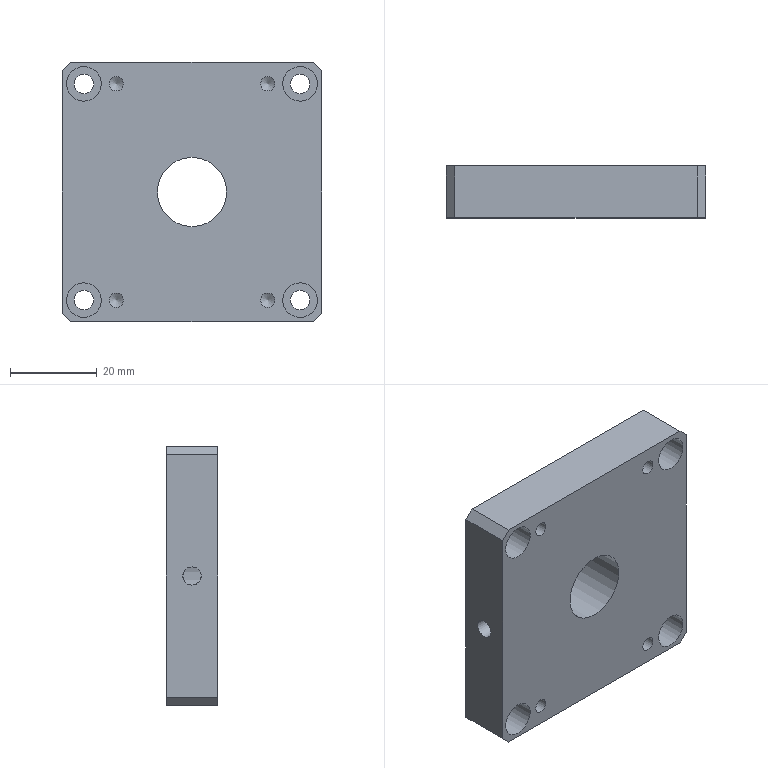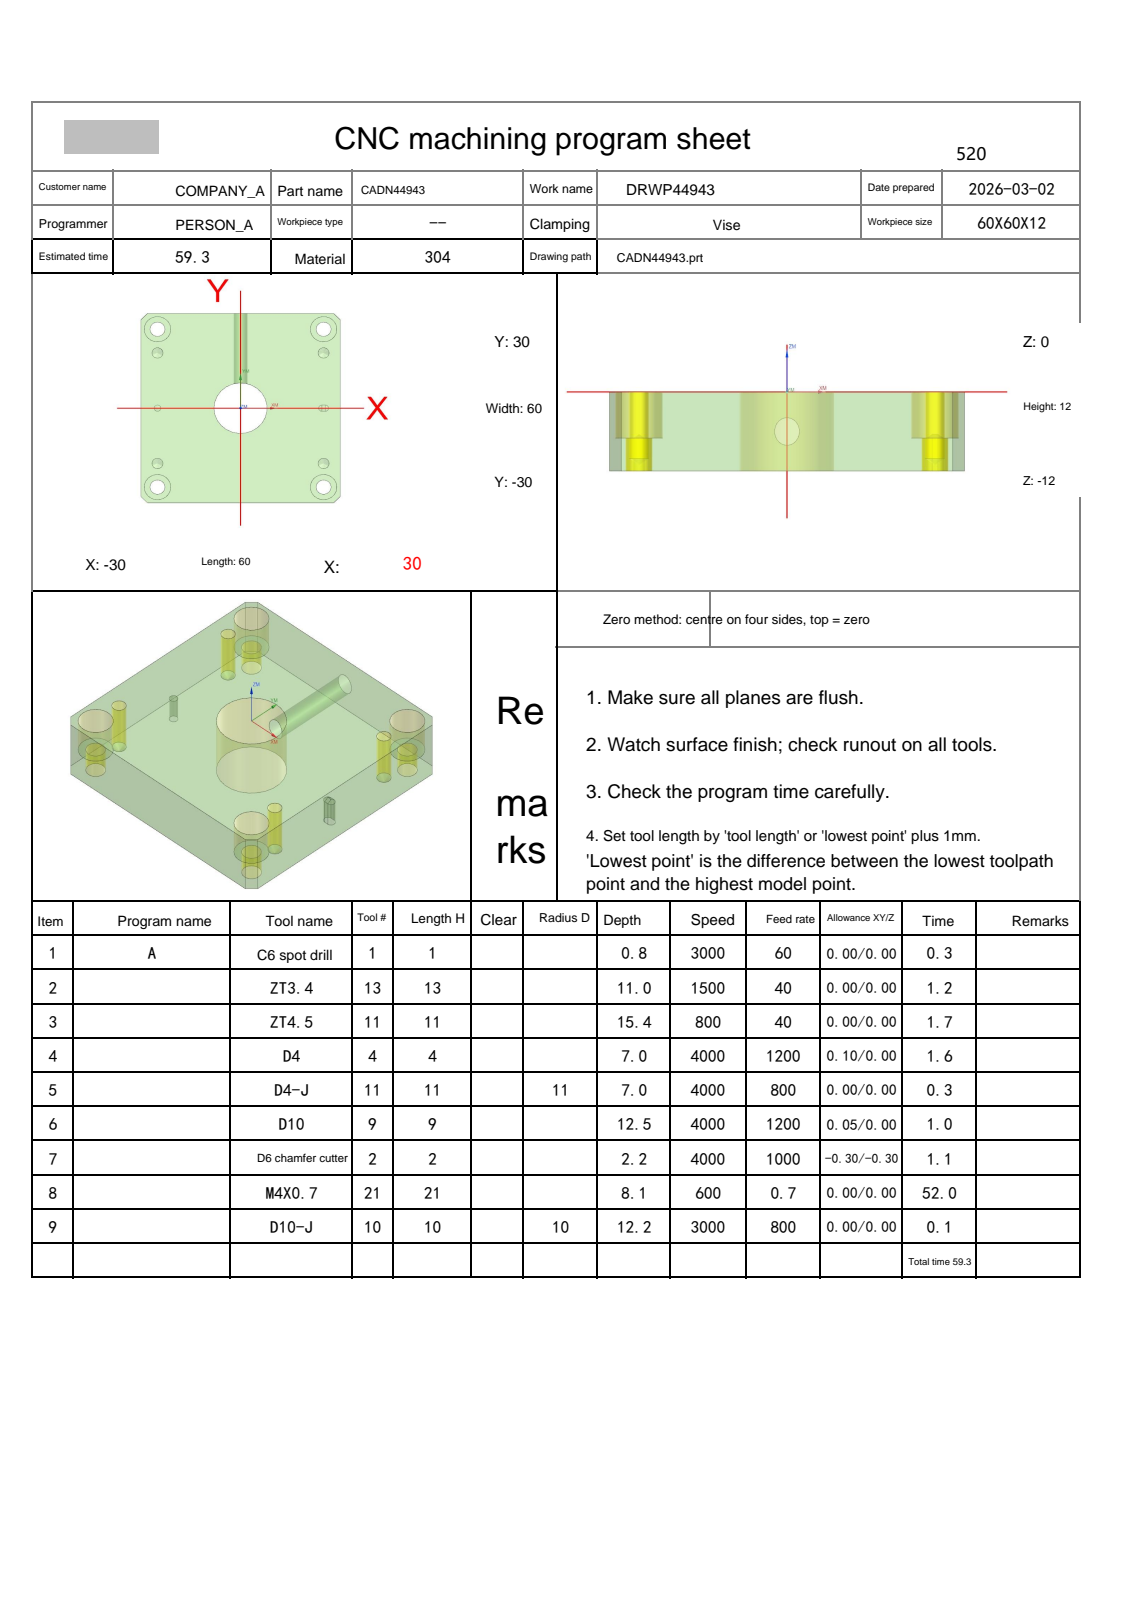NC program | NX | posted by the shop | part box 60 x 12 x 60 mm
Whole program:
%
O0001
(Machine time: 107.25 MIN)
(===Total Tool:8===)
(T1=C6 spot drill   D=6.   R=0.   D-  H01 Z=-0.8  )
(T13=ZT3.4  D=3.4  DR_a=118 D-  H13 Z=-11.  )
(T11=ZT4.5  D=4.5  DR_a=118 D-  H11 Z=-15.35)
(T4=D4      D=4.   R=0.   D-  H04 Z=-7.   )
(T9=D10     D=10.  R=0.   D-  H09 Z=-12.5 )
(T2=D6 chamfer cutter   D=6.   R=0.   D-  H02 Z=-2.2  )
(T21=M4X0.7 D=3.3  DR_a=180 D-  H21 Z=-8.1  )
(T10=D10-J  D=10.  R=0.   D10 H10 Z=-12.2 )
G80 G90 G17 G49 G40
G91 G28 Z0
M01
N1 T01 M06
(C6 spot drill  D=6. R=0. H=01 ce=0.00 di=0.00)
G00 G90 G54 X25. Y25. M03 S3000
G43 H01 Z50.
M08
G98 G81 X25. Y25. Z-.8 R1. F60.
Y17.5
Y-17.5
Y-25.
X0.0 Y0.0
X-25. Y25.
Y17.5
Y-17.5
Y-25.
G80
G00 Z50.
G91 G28 Z0.0
M05
M09
G91 G28 Z0.0
M01
N2 T13 M06
(ZT3.4 D=3.4 DR_a=118 H=13)
G00 G90 G54 X25. Y17.5 M03 S1500
G43 H13 Z50.
M08
G98 G83 X25. Y17.5 Z-11. R1. F40. Q1.
Y-17.5
X-25.
Y17.5
G80
G00 Z50.
G91 G28 Z0.0
M05
M09
G91 G28 Z0.0
M01
N3 T11 M06
(ZT4.5 D=4.5 DR_a=118 H=11)
G00 G90 G54 X-25. Y-25. M03 S800
G43 H11 Z50.
M08
G98 G83 X-25. Y-25. Z-15.352 R1. F40. Q1.
Y25.
X25.
Y-25.
G80
G00 Z50.
G91 G28 Z0.0
M05
M09
G91 G28 Z0.0
M01
N4 T04 M06
(D4  D=4. R=0. H=04 ce=0.10 di=0.00)
G00 G90 G54 X-25. Y-25. M03 S4000
G43 H04 Z50.
M08
Z.5
G03 X-25.95 Y-25.95 I0.0 J-.95 F1200.
X-25. Y-26.9 I.95 J0.0
X-25. Y-26.9 Z.3 I0.0 J1.9
X-25. Y-26.9 Z.1 I0.0 J1.9
X-25. Y-26.9 Z-.1 I0.0 J1.9
X-25. Y-26.9 Z-.3 I0.0 J1.9
X-25. Y-26.9 Z-.5 I0.0 J1.9
X-25. Y-26.9 Z-.7 I0.0 J1.9
X-25. Y-26.9 Z-.9 I0.0 J1.9
X-25. Y-26.9 Z-1.1 I0.0 J1.9
X-25. Y-26.9 Z-1.3 I0.0 J1.9
X-25. Y-26.9 Z-1.5 I0.0 J1.9
X-25. Y-26.9 Z-1.7 I0.0 J1.9
X-25. Y-26.9 Z-1.9 I0.0 J1.9
X-25. Y-26.9 Z-2.1 I0.0 J1.9
X-25. Y-26.9 Z-2.3 I0.0 J1.9
X-25. Y-26.9 Z-2.5 I0.0 J1.9
X-25. Y-26.9 Z-2.7 I0.0 J1.9
X-25. Y-26.9 Z-2.9 I0.0 J1.9
X-25. Y-26.9 Z-3.1 I0.0 J1.9
X-25. Y-26.9 Z-3.3 I0.0 J1.9
X-25. Y-26.9 Z-3.5 I0.0 J1.9
X-25. Y-26.9 Z-3.7 I0.0 J1.9
X-25. Y-26.9 Z-3.9 I0.0 J1.9
X-25. Y-26.9 Z-4.1 I0.0 J1.9
X-25. Y-26.9 Z-4.3 I0.0 J1.9
X-25. Y-26.9 Z-4.5 I0.0 J1.9
X-25. Y-26.9 Z-4.7 I0.0 J1.9
X-25. Y-26.9 Z-4.9 I0.0 J1.9
X-25. Y-26.9 Z-5.1 I0.0 J1.9
X-25. Y-26.9 Z-5.3 I0.0 J1.9
X-25. Y-26.9 Z-5.5 I0.0 J1.9
X-25. Y-26.9 Z-5.7 I0.0 J1.9
X-25. Y-26.9 Z-5.9 I0.0 J1.9
X-25. Y-26.9 Z-6.1 I0.0 J1.9
X-25. Y-26.9 Z-6.3 I0.0 J1.9
X-25. Y-26.9 Z-6.5 I0.0 J1.9
X-25. Y-26.9 Z-6.7 I0.0 J1.9
X-25. Y-26.9 Z-6.9 I0.0 J1.9
X-25. Y-23.1 Z-7. I0.0 J1.9
X-26.9 Y-25. I0.0 J-1.9
X-25. Y-26.9 I1.9 J0.0
X-23.1 Y-25. I0.0 J1.9
X-25. Y-23.1 I-1.9 J0.0
X-25.95 Y-24.05 I0.0 J-.95
X-25. Y-25. I.95 J0.0
G00 Z50.
Y25.
Z.5
G03 X-25.95 Y24.05 I0.0 J-.95
X-25. Y23.1 I.95 J0.0
X-25. Y23.1 Z.3 I0.0 J1.9
X-25. Y23.1 Z.1 I0.0 J1.9
X-25. Y23.1 Z-.1 I0.0 J1.9
X-25. Y23.1 Z-.3 I0.0 J1.9
X-25. Y23.1 Z-.5 I0.0 J1.9
X-25. Y23.1 Z-.7 I0.0 J1.9
X-25. Y23.1 Z-.9 I0.0 J1.9
X-25. Y23.1 Z-1.1 I0.0 J1.9
X-25. Y23.1 Z-1.3 I0.0 J1.9
X-25. Y23.1 Z-1.5 I0.0 J1.9
X-25. Y23.1 Z-1.7 I0.0 J1.9
X-25. Y23.1 Z-1.9 I0.0 J1.9
X-25. Y23.1 Z-2.1 I0.0 J1.9
X-25. Y23.1 Z-2.3 I0.0 J1.9
X-25. Y23.1 Z-2.5 I0.0 J1.9
X-25. Y23.1 Z-2.7 I0.0 J1.9
X-25. Y23.1 Z-2.9 I0.0 J1.9
X-25. Y23.1 Z-3.1 I0.0 J1.9
X-25. Y23.1 Z-3.3 I0.0 J1.9
X-25. Y23.1 Z-3.5 I0.0 J1.9
X-25. Y23.1 Z-3.7 I0.0 J1.9
X-25. Y23.1 Z-3.9 I0.0 J1.9
X-25. Y23.1 Z-4.1 I0.0 J1.9
X-25. Y23.1 Z-4.3 I0.0 J1.9
X-25. Y23.1 Z-4.5 I0.0 J1.9
X-25. Y23.1 Z-4.7 I0.0 J1.9
X-25. Y23.1 Z-4.9 I0.0 J1.9
X-25. Y23.1 Z-5.1 I0.0 J1.9
X-25. Y23.1 Z-5.3 I0.0 J1.9
X-25. Y23.1 Z-5.5 I0.0 J1.9
X-25. Y23.1 Z-5.7 I0.0 J1.9
X-25. Y23.1 Z-5.9 I0.0 J1.9
X-25. Y23.1 Z-6.1 I0.0 J1.9
X-25. Y23.1 Z-6.3 I0.0 J1.9
X-25. Y23.1 Z-6.5 I0.0 J1.9
X-25. Y23.1 Z-6.7 I0.0 J1.9
X-25. Y23.1 Z-6.9 I0.0 J1.9
X-25. Y26.9 Z-7. I0.0 J1.9
X-26.9 Y25. I0.0 J-1.9
X-25. Y23.1 I1.9 J0.0
X-23.1 Y25. I0.0 J1.9
X-25. Y26.9 I-1.9 J0.0
X-25.95 Y25.95 I0.0 J-.95
X-25. Y25. I.95 J0.0
G00 Z50.
X25.
Z.5
G03 X24.05 Y24.05 I0.0 J-.95
X25. Y23.1 I.95 J0.0
X25. Y23.1 Z.3 I0.0 J1.9
X25. Y23.1 Z.1 I0.0 J1.9
X25. Y23.1 Z-.1 I0.0 J1.9
X25. Y23.1 Z-.3 I0.0 J1.9
X25. Y23.1 Z-.5 I0.0 J1.9
X25. Y23.1 Z-.7 I0.0 J1.9
X25. Y23.1 Z-.9 I0.0 J1.9
X25. Y23.1 Z-1.1 I0.0 J1.9
X25. Y23.1 Z-1.3 I0.0 J1.9
X25. Y23.1 Z-1.5 I0.0 J1.9
X25. Y23.1 Z-1.7 I0.0 J1.9
X25. Y23.1 Z-1.9 I0.0 J1.9
X25. Y23.1 Z-2.1 I0.0 J1.9
X25. Y23.1 Z-2.3 I0.0 J1.9
X25. Y23.1 Z-2.5 I0.0 J1.9
X25. Y23.1 Z-2.7 I0.0 J1.9
X25. Y23.1 Z-2.9 I0.0 J1.9
X25. Y23.1 Z-3.1 I0.0 J1.9
X25. Y23.1 Z-3.3 I0.0 J1.9
X25. Y23.1 Z-3.5 I0.0 J1.9
X25. Y23.1 Z-3.7 I0.0 J1.9
X25. Y23.1 Z-3.9 I0.0 J1.9
X25. Y23.1 Z-4.1 I0.0 J1.9
X25. Y23.1 Z-4.3 I0.0 J1.9
X25. Y23.1 Z-4.5 I0.0 J1.9
X25. Y23.1 Z-4.7 I0.0 J1.9
X25. Y23.1 Z-4.9 I0.0 J1.9
X25. Y23.1 Z-5.1 I0.0 J1.9
X25. Y23.1 Z-5.3 I0.0 J1.9
X25. Y23.1 Z-5.5 I0.0 J1.9
X25. Y23.1 Z-5.7 I0.0 J1.9
X25. Y23.1 Z-5.9 I0.0 J1.9
X25. Y23.1 Z-6.1 I0.0 J1.9
X25. Y23.1 Z-6.3 I0.0 J1.9
X25. Y23.1 Z-6.5 I0.0 J1.9
X25. Y23.1 Z-6.7 I0.0 J1.9
X25. Y23.1 Z-6.9 I0.0 J1.9
X25. Y26.9 Z-7. I0.0 J1.9
X23.1 Y25. I0.0 J-1.9
X25. Y23.1 I1.9 J0.0
X26.9 Y25. I0.0 J1.9
X25. Y26.9 I-1.9 J0.0
X24.05 Y25.95 I0.0 J-.95
X25. Y25. I.95 J0.0
G00 Z50.
Y-25.
Z.5
G03 X24.05 Y-25.95 I0.0 J-.95
X25. Y-26.9 I.95 J0.0
X25. Y-26.9 Z.3 I0.0 J1.9
X25. Y-26.9 Z.1 I0.0 J1.9
X25. Y-26.9 Z-.1 I0.0 J1.9
X25. Y-26.9 Z-.3 I0.0 J1.9
X25. Y-26.9 Z-.5 I0.0 J1.9
X25. Y-26.9 Z-.7 I0.0 J1.9
X25. Y-26.9 Z-.9 I0.0 J1.9
X25. Y-26.9 Z-1.1 I0.0 J1.9
X25. Y-26.9 Z-1.3 I0.0 J1.9
X25. Y-26.9 Z-1.5 I0.0 J1.9
X25. Y-26.9 Z-1.7 I0.0 J1.9
X25. Y-26.9 Z-1.9 I0.0 J1.9
X25. Y-26.9 Z-2.1 I0.0 J1.9
X25. Y-26.9 Z-2.3 I0.0 J1.9
X25. Y-26.9 Z-2.5 I0.0 J1.9
X25. Y-26.9 Z-2.7 I0.0 J1.9
X25. Y-26.9 Z-2.9 I0.0 J1.9
X25. Y-26.9 Z-3.1 I0.0 J1.9
X25. Y-26.9 Z-3.3 I0.0 J1.9
X25. Y-26.9 Z-3.5 I0.0 J1.9
X25. Y-26.9 Z-3.7 I0.0 J1.9
X25. Y-26.9 Z-3.9 I0.0 J1.9
X25. Y-26.9 Z-4.1 I0.0 J1.9
X25. Y-26.9 Z-4.3 I0.0 J1.9
X25. Y-26.9 Z-4.5 I0.0 J1.9
X25. Y-26.9 Z-4.7 I0.0 J1.9
X25. Y-26.9 Z-4.9 I0.0 J1.9
X25. Y-26.9 Z-5.1 I0.0 J1.9
X25. Y-26.9 Z-5.3 I0.0 J1.9
X25. Y-26.9 Z-5.5 I0.0 J1.9
X25. Y-26.9 Z-5.7 I0.0 J1.9
X25. Y-26.9 Z-5.9 I0.0 J1.9
X25. Y-26.9 Z-6.1 I0.0 J1.9
X25. Y-26.9 Z-6.3 I0.0 J1.9
X25. Y-26.9 Z-6.5 I0.0 J1.9
X25. Y-26.9 Z-6.7 I0.0 J1.9
X25. Y-26.9 Z-6.9 I0.0 J1.9
X25. Y-23.1 Z-7. I0.0 J1.9
X23.1 Y-25. I0.0 J-1.9
X25. Y-26.9 I1.9 J0.0
X26.9 Y-25. I0.0 J1.9
X25. Y-23.1 I-1.9 J0.0
X24.05 Y-24.05 I0.0 J-.95
X25. Y-25. I.95 J0.0
G00 Z50.
G91 G28 Z0.0
M05
M09
G91 G28 Z0.0
M01
N5 T11 M06
(D4-J  D=4. R=0. H=11 ce=0.00 di=0.00)
G00 G90 G54 X-25. Y-25. M03 S4000
G43 H11 Z50.
M08
Z.5
G41 D11
G01 X-25.196 Y-25.04 F800.
G03 X-25.99 Y-26.01 I.196 J-.97
X-25. Y-27. I.99 J0.0
X-25. Y-27. Z-4.5 I0.0 J2.
X-25. Y-23. Z-7. I0.0 J2.
X-27. Y-25. I0.0 J-2.
X-25. Y-27. I2. J0.0
X-23. Y-25. I0.0 J2.
X-25. Y-23. I-2. J0.0
X-25.99 Y-23.99 I0.0 J-.99
X-25.196 Y-24.96 I.99 J0.0
G01 G40 X-25. Y-25.
G00 Z50.
Y25.
Z.5
G41 D11
G01 X-25.196 Y24.96
G03 X-25.99 Y23.99 I.196 J-.97
X-25. Y23. I.99 J0.0
X-25. Y23. Z-4.5 I0.0 J2.
X-25. Y27. Z-7. I0.0 J2.
X-27. Y25. I0.0 J-2.
X-25. Y23. I2. J0.0
X-23. Y25. I0.0 J2.
X-25. Y27. I-2. J0.0
X-25.99 Y26.01 I0.0 J-.99
X-25.196 Y25.04 I.99 J0.0
G01 G40 X-25. Y25.
G00 Z50.
X25.
Z.5
G41 D11
G01 X24.804 Y24.96
G03 X24.01 Y23.99 I.196 J-.97
X25. Y23. I.99 J0.0
X25. Y23. Z-4.5 I0.0 J2.
X25. Y27. Z-7. I0.0 J2.
X23. Y25. I0.0 J-2.
X25. Y23. I2. J0.0
X27. Y25. I0.0 J2.
X25. Y27. I-2. J0.0
X24.01 Y26.01 I0.0 J-.99
X24.804 Y25.04 I.99 J0.0
G01 G40 X25. Y25.
G00 Z50.
Y-25.
Z.5
G41 D11
G01 X24.804 Y-25.04
G03 X24.01 Y-26.01 I.196 J-.97
X25. Y-27. I.99 J0.0
X25. Y-27. Z-4.5 I0.0 J2.
X25. Y-23. Z-7. I0.0 J2.
X23. Y-25. I0.0 J-2.
X25. Y-27. I2. J0.0
X27. Y-25. I0.0 J2.
X25. Y-23. I-2. J0.0
X24.01 Y-23.99 I0.0 J-.99
X24.804 Y-24.96 I.99 J0.0
G01 G40 X25. Y-25.
G00 Z50.
G91 G28 Z0.0
M05
M09
G91 G28 Z0.0
M01
N6 T09 M06
(D10  D=10. R=0. H=09 ce=0.05 di=0.00)
G00 G90 G54 X0.0 Y0.0 M03 S4000
G43 H09 Z50.
M08
Z.5
G03 X-1.475 Y-1.475 I0.0 J-1.475 F1200.
X0.0 Y-2.95 I1.475 J0.0
X0.0 Y-2.95 Z.3 I0.0 J2.95
X0.0 Y-2.95 Z.1 I0.0 J2.95
X0.0 Y-2.95 Z-.1 I0.0 J2.95
X0.0 Y-2.95 Z-.3 I0.0 J2.95
X0.0 Y-2.95 Z-.5 I0.0 J2.95
X0.0 Y-2.95 Z-.7 I0.0 J2.95
X0.0 Y-2.95 Z-.9 I0.0 J2.95
X0.0 Y-2.95 Z-1.1 I0.0 J2.95
X0.0 Y-2.95 Z-1.3 I0.0 J2.95
X0.0 Y-2.95 Z-1.5 I0.0 J2.95
X0.0 Y-2.95 Z-1.7 I0.0 J2.95
X0.0 Y-2.95 Z-1.9 I0.0 J2.95
X0.0 Y-2.95 Z-2.1 I0.0 J2.95
X0.0 Y-2.95 Z-2.3 I0.0 J2.95
X0.0 Y-2.95 Z-2.5 I0.0 J2.95
X0.0 Y-2.95 Z-2.7 I0.0 J2.95
X0.0 Y-2.95 Z-2.9 I0.0 J2.95
X0.0 Y-2.95 Z-3.1 I0.0 J2.95
X0.0 Y-2.95 Z-3.3 I0.0 J2.95
X0.0 Y-2.95 Z-3.5 I0.0 J2.95
X0.0 Y-2.95 Z-3.7 I0.0 J2.95
X0.0 Y-2.95 Z-3.9 I0.0 J2.95
X0.0 Y-2.95 Z-4.1 I0.0 J2.95
X0.0 Y-2.95 Z-4.3 I0.0 J2.95
X0.0 Y-2.95 Z-4.5 I0.0 J2.95
X0.0 Y-2.95 Z-4.7 I0.0 J2.95
X0.0 Y-2.95 Z-4.9 I0.0 J2.95
X0.0 Y-2.95 Z-5.1 I0.0 J2.95
X0.0 Y-2.95 Z-5.3 I0.0 J2.95
X0.0 Y-2.95 Z-5.5 I0.0 J2.95
X0.0 Y-2.95 Z-5.7 I0.0 J2.95
X0.0 Y-2.95 Z-5.9 I0.0 J2.95
X0.0 Y-2.95 Z-6.1 I0.0 J2.95
X0.0 Y-2.95 Z-6.3 I0.0 J2.95
X0.0 Y-2.95 Z-6.5 I0.0 J2.95
X0.0 Y-2.95 Z-6.7 I0.0 J2.95
X0.0 Y-2.95 Z-6.9 I0.0 J2.95
X0.0 Y-2.95 Z-7.1 I0.0 J2.95
X0.0 Y-2.95 Z-7.3 I0.0 J2.95
X0.0 Y-2.95 Z-7.5 I0.0 J2.95
X0.0 Y-2.95 Z-7.7 I0.0 J2.95
X0.0 Y-2.95 Z-7.9 I0.0 J2.95
X0.0 Y-2.95 Z-8.1 I0.0 J2.95
X0.0 Y-2.95 Z-8.3 I0.0 J2.95
X0.0 Y-2.95 Z-8.5 I0.0 J2.95
X0.0 Y-2.95 Z-8.7 I0.0 J2.95
X0.0 Y-2.95 Z-8.9 I0.0 J2.95
X0.0 Y-2.95 Z-9.1 I0.0 J2.95
X0.0 Y-2.95 Z-9.3 I0.0 J2.95
X0.0 Y-2.95 Z-9.5 I0.0 J2.95
X0.0 Y-2.95 Z-9.7 I0.0 J2.95
X0.0 Y-2.95 Z-9.9 I0.0 J2.95
X0.0 Y-2.95 Z-10.1 I0.0 J2.95
X0.0 Y-2.95 Z-10.3 I0.0 J2.95
X0.0 Y-2.95 Z-10.5 I0.0 J2.95
X0.0 Y-2.95 Z-10.7 I0.0 J2.95
X0.0 Y-2.95 Z-10.9 I0.0 J2.95
X0.0 Y-2.95 Z-11.1 I0.0 J2.95
X0.0 Y-2.95 Z-11.3 I0.0 J2.95
X0.0 Y-2.95 Z-11.5 I0.0 J2.95
X0.0 Y-2.95 Z-11.7 I0.0 J2.95
X0.0 Y-2.95 Z-11.9 I0.0 J2.95
X0.0 Y-2.95 Z-12.1 I0.0 J2.95
X0.0 Y-2.95 Z-12.3 I0.0 J2.95
X0.0 Y-2.95 Z-12.5 I0.0 J2.95
X2.95 Y0.0 I0.0 J2.95
X0.0 Y2.95 I-2.95 J0.0
X-2.95 Y0.0 I0.0 J-2.95
X0.0 Y-2.95 I2.95 J0.0
X1.475 Y-1.475 I0.0 J1.475
X0.0 Y0.0 I-1.475 J0.0
G00 Z50.
G91 G28 Z0.0
M05
M09
G91 G28 Z0.0
M01
N7 T02 M06
(D6 chamfer cutter  D=6. R=0. H=02 ce=0.00 di=0.00)
G00 G90 G54 X25. Y17.5 M03 S4000
G43 H02 Z50.
M08
G98 G81 X25. Y17.5 Z-2.2 R3. F80.
Y-17.5
X-25.
Y17.5
G80
G00 Z50.
G00 G90 X21.788 Y24.253 M03 S4000
Z50.
Z2.5
G01 X21.84 Y24.038 Z2.42 F500.
X21.976 Y23.672 Z2.278
X22.153 Y23.325 Z2.136
X22.371 Y23.001 Z1.994
X22.625 Y22.705 Z1.852
X22.912 Y22.441 Z1.71
X23.228 Y22.212 Z1.568
X23.472 Y22.072 Z1.465
X23.828 Y21.912 Z1.323
X24.2 Y21.795 Z1.181
X24.584 Y21.723 Z1.039
X24.973 Y21.697 Z.897
X25.362 Y21.717 Z.755
X25.747 Y21.783 Z.613
X26.121 Y21.893 Z.471
X26.48 Y22.047 Z.329
X26.818 Y22.242 Z.187
X27.13 Y22.476 Z.045
X27.413 Y22.744 Z-.097
X27.662 Y23.045 Z-.239
X27.874 Y23.372 Z-.381
X28.046 Y23.722 Z-.523
X28.175 Y24.09 Z-.665
X28.26 Y24.471 Z-.807
X28.3 Y24.859 Z-.949
Y25. Z-1.
G03 X25. Y28.3 I-3.3 J0.0
X21.7 Y25. I0.0 J-3.3
X25. Y21.7 I3.3 J0.0
X28.3 Y25. I0.0 J3.3
X28.262 Y25.498 I-3.3 J0.0
G01 Z1.5
G00 Z50.
X21.788 Y-25.747
Z2.5
G01 X21.84 Y-25.962 Z2.42
X21.976 Y-26.328 Z2.278
X22.153 Y-26.675 Z2.136
X22.371 Y-26.999 Z1.994
X22.625 Y-27.295 Z1.852
X22.912 Y-27.559 Z1.71
X23.228 Y-27.788 Z1.568
X23.472 Y-27.928 Z1.465
X23.828 Y-28.088 Z1.323
X24.2 Y-28.205 Z1.181
X24.584 Y-28.277 Z1.039
X24.973 Y-28.303 Z.897
X25.362 Y-28.283 Z.755
X25.747 Y-28.217 Z.613
X26.121 Y-28.107 Z.471
X26.48 Y-27.953 Z.329
X26.818 Y-27.758 Z.187
X27.13 Y-27.524 Z.045
X27.413 Y-27.256 Z-.097
X27.662 Y-26.955 Z-.239
X27.874 Y-26.628 Z-.381
X28.046 Y-26.278 Z-.523
X28.175 Y-25.91 Z-.665
X28.26 Y-25.529 Z-.807
X28.3 Y-25.141 Z-.949
Y-25. Z-1.
G03 X25. Y-21.7 I-3.3 J0.0
X21.7 Y-25. I0.0 J-3.3
X25. Y-28.3 I3.3 J0.0
X28.3 Y-25. I0.0 J3.3
X28.262 Y-24.502 I-3.3 J0.0
G01 Z1.5
G00 Z50.
X-28.212 Y-25.747
Z2.5
G01 X-28.16 Y-25.962 Z2.42
X-28.024 Y-26.328 Z2.278
X-27.847 Y-26.675 Z2.136
X-27.629 Y-26.999 Z1.994
X-27.375 Y-27.295 Z1.852
X-27.088 Y-27.559 Z1.71
X-26.772 Y-27.788 Z1.568
X-26.528 Y-27.928 Z1.465
X-26.172 Y-28.088 Z1.323
X-25.8 Y-28.205 Z1.181
X-25.416 Y-28.277 Z1.039
X-25.027 Y-28.303 Z.897
X-24.638 Y-28.283 Z.755
X-24.253 Y-28.217 Z.613
X-23.879 Y-28.107 Z.471
X-23.52 Y-27.953 Z.329
X-23.182 Y-27.758 Z.187
X-22.87 Y-27.524 Z.045
X-22.587 Y-27.256 Z-.097
X-22.338 Y-26.955 Z-.239
X-22.126 Y-26.628 Z-.381
X-21.954 Y-26.278 Z-.523
X-21.825 Y-25.91 Z-.665
X-21.74 Y-25.529 Z-.807
X-21.7 Y-25.141 Z-.949
Y-25. Z-1.
G03 X-25. Y-21.7 I-3.3 J0.0
X-28.3 Y-25. I0.0 J-3.3
X-25. Y-28.3 I3.3 J0.0
X-21.7 Y-25. I0.0 J3.3
X-21.738 Y-24.502 I-3.3 J0.0
G01 Z1.5
G00 Z50.
X-28.212 Y24.253
Z2.5
G01 X-28.16 Y24.038 Z2.42
X-28.024 Y23.672 Z2.278
X-27.847 Y23.325 Z2.136
X-27.629 Y23.001 Z1.994
X-27.375 Y22.705 Z1.852
X-27.088 Y22.441 Z1.71
X-26.772 Y22.212 Z1.568
X-26.528 Y22.072 Z1.465
X-26.172 Y21.912 Z1.323
X-25.8 Y21.795 Z1.181
X-25.416 Y21.723 Z1.039
X-25.027 Y21.697 Z.897
X-24.638 Y21.717 Z.755
X-24.253 Y21.783 Z.613
X-23.879 Y21.893 Z.471
X-23.52 Y22.047 Z.329
X-23.182 Y22.242 Z.187
X-22.87 Y22.476 Z.045
X-22.587 Y22.744 Z-.097
X-22.338 Y23.045 Z-.239
X-22.126 Y23.372 Z-.381
X-21.954 Y23.722 Z-.523
X-21.825 Y24.09 Z-.665
X-21.74 Y24.471 Z-.807
X-21.7 Y24.859 Z-.949
Y25. Z-1.
G03 X-25. Y28.3 I-3.3 J0.0
X-28.3 Y25. I0.0 J-3.3
X-25. Y21.7 I3.3 J0.0
X-21.7 Y25. I0.0 J3.3
X-21.738 Y25.498 I-3.3 J0.0
G01 Z1.5
G00 Z50.
G00 G90 X31.227 Y.386 M03 S3500
Z50.
Z.172
G01 Z-1.2 F1000.
G03 X31.027 Y.1 I1.532 J-1.286
G01 X30.997 Y.054
X31. Y0.0
Y-28.
X30.966 Y-28.259
X30.866 Y-28.5
X30.707 Y-28.707
X28.707 Y-30.707
X28.5 Y-30.866
X28.259 Y-30.966
X28. Y-31.
X-28.
X-28.259 Y-30.966
X-28.5 Y-30.866
X-28.707 Y-30.707
X-30.707 Y-28.707
X-30.866 Y-28.5
X-30.966 Y-28.259
X-31. Y-28.
Y28.
X-30.966 Y28.259
X-30.866 Y28.5
X-30.707 Y28.707
X-28.707 Y30.707
X-28.5 Y30.866
X-28.259 Y30.966
X-28. Y31.
X28.
X28.259 Y30.966
X28.5 Y30.866
X28.707 Y30.707
X30.707 Y28.707
X30.866 Y28.5
X30.966 Y28.259
X31. Y28.
Y0.0
X30.997 Y-.054
X31.027 Y-.1
G03 X31.227 Y-.386 I1.732 J1.
G01 Z.172
G00 Z10.
X22.197 Y25.401
Z.233
G01 Z-1.2
G03 X22.019 Y25.102 I1.624 J-1.167
G01 X21.993 Y25.054
X22. Y25.
G03 X25. Y22. I3. J0.0
X28. Y25. I0.0 J3.
X25. Y28. I-3. J0.0
X22. Y25. I0.0 J-3.
G01 X21.993 Y24.946
X22.019 Y24.898
G03 X22.197 Y24.599 I1.802 J.868
G01 Z.233
G00 Z2.55
X24.506 Y17.919
Z.405
G01 Z-1.2
G03 X24.359 Y17.603 I1.732 J-1.
G01 X24.338 Y17.553
X24.35 Y17.5
G03 X25. Y16.85 I.65 J0.0
X25.65 Y17.5 I0.0 J.65
X25. Y18.15 I-.65 J0.0
X24.35 Y17.5 I0.0 J-.65
G01 X24.338 Y17.447
X24.359 Y17.397
G03 X24.506 Y17.081 I1.879 J.684
G01 Z.405
G00 Z10.
Y-17.081
Z.405
G01 Z-1.2
G03 X24.359 Y-17.397 I1.732 J-1.
G01 X24.338 Y-17.447
X24.35 Y-17.5
G03 X25. Y-18.15 I.65 J0.0
X25.65 Y-17.5 I0.0 J.65
X25. Y-16.85 I-.65 J0.0
X24.35 Y-17.5 I0.0 J-.65
G01 X24.338 Y-17.553
X24.359 Y-17.603
G03 X24.506 Y-17.919 I1.879 J.684
G01 Z.405
G00 Z2.55
X22.197 Y-24.599
Z.233
G01 Z-1.2
G03 X22.019 Y-24.898 I1.624 J-1.167
G01 X21.993 Y-24.946
X22. Y-25.
G03 X25. Y-28. I3. J0.0
X28. Y-25. I0.0 J3.
X25. Y-22. I-3. J0.0
X22. Y-25. I0.0 J-3.
G01 X21.993 Y-25.054
X22.019 Y-25.102
G03 X22.197 Y-25.401 I1.802 J.868
G01 Z.233
G00 Z10.
X6.794 Y-.397
Z.208
G01 Z-1.2
G03 X6.978 Y-.101 I-1.597 J1.204
G01 X7.006 Y-.054
X7. Y0.0
G03 X0.0 Y7. I-7. J0.0
X-7. Y0.0 I0.0 J-7.
X0.0 Y-7. I7. J0.0
X7. Y0.0 I0.0 J7.
G01 X7.006 Y.054
X6.978 Y.101
G03 X6.794 Y.397 I-1.782 J-.908
G01 Z.208
G00 Z10.
X-27.803 Y-24.599
Z.233
G01 Z-1.2
G03 X-27.981 Y-24.898 I1.624 J-1.167
G01 X-28.007 Y-24.946
X-28. Y-25.
G03 X-25. Y-28. I3. J0.0
X-22. Y-25. I0.0 J3.
X-25. Y-22. I-3. J0.0
X-28. Y-25. I0.0 J-3.
G01 X-28.007 Y-25.054
X-27.981 Y-25.102
G03 X-27.803 Y-25.401 I1.802 J.868
G01 Z.233
G00 Z2.55
X-25.494 Y-17.081
Z.405
G01 Z-1.2
G03 X-25.641 Y-17.397 I1.732 J-1.
G01 X-25.662 Y-17.447
X-25.65 Y-17.5
G03 X-25. Y-18.15 I.65 J0.0
X-24.35 Y-17.5 I0.0 J.65
X-25. Y-16.85 I-.65 J0.0
X-25.65 Y-17.5 I0.0 J-.65
G01 X-25.662 Y-17.553
X-25.641 Y-17.603
G03 X-25.494 Y-17.919 I1.879 J.684
G01 Z.405
G00 Z10.
Y17.919
Z.405
G01 Z-1.2
G03 X-25.641 Y17.603 I1.732 J-1.
G01 X-25.662 Y17.553
X-25.65 Y17.5
G03 X-25. Y16.85 I.65 J0.0
X-24.35 Y17.5 I0.0 J.65
X-25. Y18.15 I-.65 J0.0
X-25.65 Y17.5 I0.0 J-.65
G01 X-25.662 Y17.447
X-25.641 Y17.397
G03 X-25.494 Y17.081 I1.879 J.684
G01 Z.405
G00 Z2.55
X-27.803 Y25.401
Z.233
G01 Z-1.2
G03 X-27.981 Y25.102 I1.624 J-1.167
G01 X-28.007 Y25.054
X-28. Y25.
G03 X-25. Y22. I3. J0.0
X-22. Y25. I0.0 J3.
X-25. Y28. I-3. J0.0
X-28. Y25. I0.0 J-3.
G01 X-28.007 Y24.946
X-27.981 Y24.898
G03 X-27.803 Y24.599 I1.802 J.868
G01 Z.233
G00 Z50.
G91 G28 Z0.0
M05
M09
G91 G28 Z0.0
M01
N8 T21 M06
(M4X0.7 D=3.3 DR_a=180 H=21)
G00 G90 G54 X25. Y17.5 M03 S600
G43 H21 Z50.
M08
G95
G98 G84 X25. Y17.5 Z-8.1 R1. F.7 Q1.
Y-17.5
X-25.
Y17.5
G80
G94
G00 Z50.
G91 G28 Z0.0
M05
M09
G91 G28 Z0.0
M01
N9 T10 M06
(D10-J  D=10. R=0. H=10 ce=0.00 di=0.00)
G00 G90 G54 X-.199 Y-1.5 M03 S3000
G43 H10 Z10.
M08
Z-4.6
G01 Z-6.1 F800.
G41 D10
X1.5
G03 X3. Y0.0 I0.0 J1.5
X0.0 Y3. I-3. J0.0
X-3. Y0.0 I0.0 J-3.
X0.0 Y-3. I3. J0.0
X3. Y0.0 I0.0 J3.
X2.973 Y.399 I-3. J0.0
X1.487 Y1.699 I-1.487 J-.199
G01 X1.287 Y1.686
X-.199 Y1.487
G40 X-.398 Y1.46
Z-4.6
G00 X-.199 Y-1.5
Z-10.7
G01 Z-12.2
G41 D10
X1.5
G03 X3. Y0.0 I0.0 J1.5
X0.0 Y3. I-3. J0.0
X-3. Y0.0 I0.0 J-3.
X0.0 Y-3. I3. J0.0
X3. Y0.0 I0.0 J3.
X2.973 Y.399 I-3. J0.0
X1.487 Y1.699 I-1.487 J-.199
G01 X1.287 Y1.686
X-.199 Y1.487
G40 X-.398 Y1.46
Z-10.7
G00 Z10.
M05
M09
G91 G28 Z0.0
G91 G28 Y0.0
M30
%